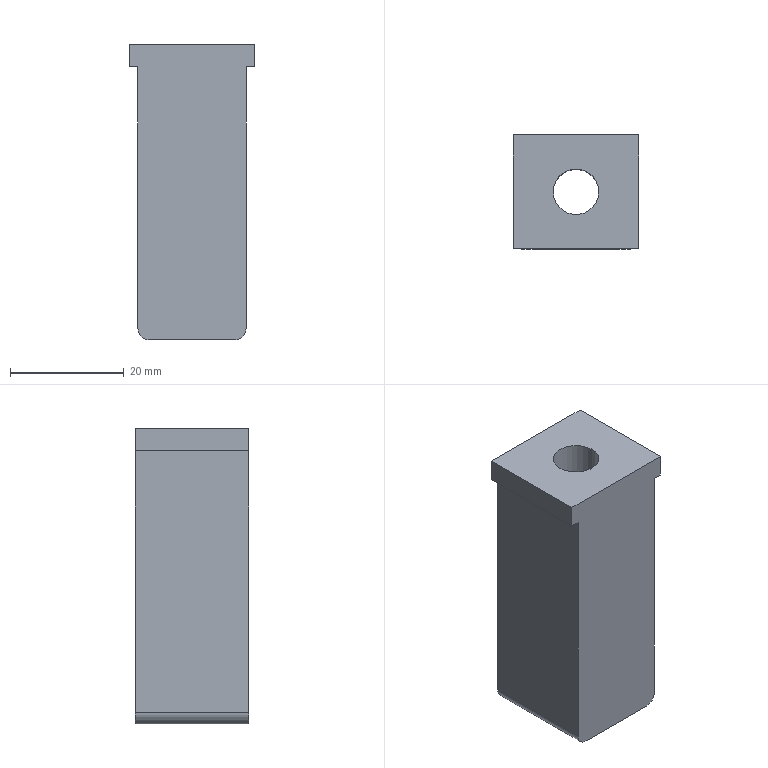Part | NX | features EXTRUDE 3, DATUM_CSYS 2, BLEND 1, SKETCH 1 | 1 solid | 13 faces | box 22 x 20 x 52 mm | volume 17352 mm3 | plane 10 | cylinder 3 | commonest cylinder face diameters 4 x2 8 x1
STEP:
#1=CARTESIAN_POINT('',(9.5,-10.,-50.));
#2=VERTEX_POINT('',#1);
#3=CARTESIAN_POINT('',(9.5,-10.,-4.));
#4=VERTEX_POINT('',#3);
#5=CARTESIAN_POINT('',(9.5,-10.,-52.));
#6=DIRECTION('',(0.,0.,1.));
#7=VECTOR('',#6,1000.);
#8=LINE('',#5,#7);
#9=EDGE_CURVE('',#2,#4,#8,.T.);
#10=ORIENTED_EDGE('',*,*,#9,.F.);
#11=CARTESIAN_POINT('',(9.5,10.,-50.));
#12=VERTEX_POINT('',#11);
#13=CARTESIAN_POINT('',(9.5,10.,-50.));
#14=DIRECTION('',(0.,1.,0.));
#15=VECTOR('',#14,1000.);
#16=LINE('',#13,#15);
#17=EDGE_CURVE('',#2,#12,#16,.T.);
#18=ORIENTED_EDGE('',*,*,#17,.T.);
#19=CARTESIAN_POINT('',(9.5,10.,-4.));
#20=VERTEX_POINT('',#19);
#21=CARTESIAN_POINT('',(9.5,10.,-52.));
#22=DIRECTION('',(0.,0.,1.));
#23=VECTOR('',#22,1000.);
#24=LINE('',#21,#23);
#25=EDGE_CURVE('',#12,#20,#24,.T.);
#26=ORIENTED_EDGE('',*,*,#25,.T.);
#27=CARTESIAN_POINT('',(9.5,-10.,-4.));
#28=DIRECTION('',(0.,1.,0.));
#29=VECTOR('',#28,1000.);
#30=LINE('',#27,#29);
#31=EDGE_CURVE('',#4,#20,#30,.T.);
#32=ORIENTED_EDGE('',*,*,#31,.F.);
#33=EDGE_LOOP('',(#10,#18,#26,#32));
#34=FACE_BOUND('',#33,.T.);
#35=CARTESIAN_POINT('',(9.5,-10.,-52.));
#36=DIRECTION('',(1.,0.,0.));
#37=DIRECTION('',(0.,0.,-1.));
#38=AXIS2_PLACEMENT_3D('',#35,#36,#37);
#39=PLANE('',#38);
#40=ADVANCED_FACE('',(#34),#39,.T.);
#41=ORIENTED_EDGE('',*,*,#25,.F.);
#42=CARTESIAN_POINT('',(7.5,10.,-52.));
#43=VERTEX_POINT('',#42);
#44=CARTESIAN_POINT('',(7.5,10.,-50.));
#45=DIRECTION('',(0.,1.,0.));
#46=DIRECTION('',(0.,0.,1.));
#47=AXIS2_PLACEMENT_3D('',#44,#45,#46);
#48=CIRCLE('',#47,2.);
#49=EDGE_CURVE('',#12,#43,#48,.T.);
#50=ORIENTED_EDGE('',*,*,#49,.T.);
#51=CARTESIAN_POINT('',(-7.5,10.,-52.));
#52=VERTEX_POINT('',#51);
#53=CARTESIAN_POINT('',(9.5,10.,-52.));
#54=DIRECTION('',(-1.,0.,0.));
#55=VECTOR('',#54,1000.);
#56=LINE('',#53,#55);
#57=EDGE_CURVE('',#43,#52,#56,.T.);
#58=ORIENTED_EDGE('',*,*,#57,.T.);
#59=CARTESIAN_POINT('',(-9.5,10.,-50.));
#60=VERTEX_POINT('',#59);
#61=CARTESIAN_POINT('',(-7.5,10.,-50.));
#62=DIRECTION('',(0.,1.,0.));
#63=DIRECTION('',(0.,0.,1.));
#64=AXIS2_PLACEMENT_3D('',#61,#62,#63);
#65=CIRCLE('',#64,2.);
#66=EDGE_CURVE('',#52,#60,#65,.T.);
#67=ORIENTED_EDGE('',*,*,#66,.T.);
#68=CARTESIAN_POINT('',(-9.5,10.,-4.));
#69=VERTEX_POINT('',#68);
#70=CARTESIAN_POINT('',(-9.5,10.,-52.));
#71=DIRECTION('',(0.,0.,1.));
#72=VECTOR('',#71,1000.);
#73=LINE('',#70,#72);
#74=EDGE_CURVE('',#60,#69,#73,.T.);
#75=ORIENTED_EDGE('',*,*,#74,.T.);
#76=CARTESIAN_POINT('',(-11.,10.,-4.));
#77=VERTEX_POINT('',#76);
#78=CARTESIAN_POINT('',(9.5,10.,-4.));
#79=DIRECTION('',(1.,0.,0.));
#80=VECTOR('',#79,1000.);
#81=LINE('',#78,#80);
#82=EDGE_CURVE('',#77,#69,#81,.T.);
#83=ORIENTED_EDGE('',*,*,#82,.F.);
#84=CARTESIAN_POINT('',(-11.,10.,0.));
#85=VERTEX_POINT('',#84);
#86=CARTESIAN_POINT('',(-11.,10.,-4.));
#87=DIRECTION('',(0.,0.,1.));
#88=VECTOR('',#87,1000.);
#89=LINE('',#86,#88);
#90=EDGE_CURVE('',#77,#85,#89,.T.);
#91=ORIENTED_EDGE('',*,*,#90,.T.);
#92=CARTESIAN_POINT('',(11.,10.,0.));
#93=VERTEX_POINT('',#92);
#94=CARTESIAN_POINT('',(9.5,10.,0.));
#95=DIRECTION('',(-1.,0.,0.));
#96=VECTOR('',#95,1000.);
#97=LINE('',#94,#96);
#98=EDGE_CURVE('',#93,#85,#97,.T.);
#99=ORIENTED_EDGE('',*,*,#98,.F.);
#100=CARTESIAN_POINT('',(11.,10.,-4.));
#101=VERTEX_POINT('',#100);
#102=CARTESIAN_POINT('',(11.,10.,-4.));
#103=DIRECTION('',(0.,0.,1.));
#104=VECTOR('',#103,1000.);
#105=LINE('',#102,#104);
#106=EDGE_CURVE('',#101,#93,#105,.T.);
#107=ORIENTED_EDGE('',*,*,#106,.F.);
#108=CARTESIAN_POINT('',(9.5,10.,-4.));
#109=DIRECTION('',(1.,0.,0.));
#110=VECTOR('',#109,1000.);
#111=LINE('',#108,#110);
#112=EDGE_CURVE('',#20,#101,#111,.T.);
#113=ORIENTED_EDGE('',*,*,#112,.F.);
#114=EDGE_LOOP('',(#41,#50,#58,#67,#75,#83,#91,#99,#107,#113));
#115=FACE_BOUND('',#114,.T.);
#116=CARTESIAN_POINT('',(9.5,10.,-52.));
#117=DIRECTION('',(0.,1.,0.));
#118=DIRECTION('',(0.,0.,1.));
#119=AXIS2_PLACEMENT_3D('',#116,#117,#118);
#120=PLANE('',#119);
#121=ADVANCED_FACE('',(#115),#120,.T.);
#122=ORIENTED_EDGE('',*,*,#74,.F.);
#123=CARTESIAN_POINT('',(-9.5,-10.,-50.));
#124=VERTEX_POINT('',#123);
#125=CARTESIAN_POINT('',(-9.5,-10.,-50.));
#126=DIRECTION('',(0.,-1.,0.));
#127=VECTOR('',#126,1000.);
#128=LINE('',#125,#127);
#129=EDGE_CURVE('',#60,#124,#128,.T.);
#130=ORIENTED_EDGE('',*,*,#129,.T.);
#131=CARTESIAN_POINT('',(-9.5,-10.,-4.));
#132=VERTEX_POINT('',#131);
#133=CARTESIAN_POINT('',(-9.5,-10.,-52.));
#134=DIRECTION('',(0.,0.,1.));
#135=VECTOR('',#134,1000.);
#136=LINE('',#133,#135);
#137=EDGE_CURVE('',#124,#132,#136,.T.);
#138=ORIENTED_EDGE('',*,*,#137,.T.);
#139=CARTESIAN_POINT('',(-9.5,10.,-4.));
#140=DIRECTION('',(0.,-1.,0.));
#141=VECTOR('',#140,1000.);
#142=LINE('',#139,#141);
#143=EDGE_CURVE('',#69,#132,#142,.T.);
#144=ORIENTED_EDGE('',*,*,#143,.F.);
#145=EDGE_LOOP('',(#122,#130,#138,#144));
#146=FACE_BOUND('',#145,.T.);
#147=CARTESIAN_POINT('',(-9.5,10.,-52.));
#148=DIRECTION('',(-1.,0.,0.));
#149=DIRECTION('',(0.,0.,1.));
#150=AXIS2_PLACEMENT_3D('',#147,#148,#149);
#151=PLANE('',#150);
#152=ADVANCED_FACE('',(#146),#151,.T.);
#153=CARTESIAN_POINT('',(-7.5,-10.,-52.));
#154=VERTEX_POINT('',#153);
#155=CARTESIAN_POINT('',(7.5,-10.,-52.));
#156=VERTEX_POINT('',#155);
#157=CARTESIAN_POINT('',(-9.5,-10.,-52.));
#158=DIRECTION('',(1.,0.,0.));
#159=VECTOR('',#158,1000.);
#160=LINE('',#157,#159);
#161=EDGE_CURVE('',#154,#156,#160,.T.);
#162=ORIENTED_EDGE('',*,*,#161,.T.);
#163=CARTESIAN_POINT('',(7.5,-10.,-50.));
#164=DIRECTION('',(0.,-1.,0.));
#165=DIRECTION('',(1.,0.,0.));
#166=AXIS2_PLACEMENT_3D('',#163,#164,#165);
#167=CIRCLE('',#166,2.);
#168=EDGE_CURVE('',#156,#2,#167,.T.);
#169=ORIENTED_EDGE('',*,*,#168,.T.);
#170=ORIENTED_EDGE('',*,*,#9,.T.);
#171=CARTESIAN_POINT('',(11.,-10.,-4.));
#172=VERTEX_POINT('',#171);
#173=CARTESIAN_POINT('',(11.,-10.,-4.));
#174=DIRECTION('',(-1.,0.,0.));
#175=VECTOR('',#174,1000.);
#176=LINE('',#173,#175);
#177=EDGE_CURVE('',#172,#4,#176,.T.);
#178=ORIENTED_EDGE('',*,*,#177,.F.);
#179=CARTESIAN_POINT('',(11.,-10.,0.));
#180=VERTEX_POINT('',#179);
#181=CARTESIAN_POINT('',(11.,-10.,-4.));
#182=DIRECTION('',(0.,0.,1.));
#183=VECTOR('',#182,1000.);
#184=LINE('',#181,#183);
#185=EDGE_CURVE('',#172,#180,#184,.T.);
#186=ORIENTED_EDGE('',*,*,#185,.T.);
#187=CARTESIAN_POINT('',(-11.,-10.,0.));
#188=VERTEX_POINT('',#187);
#189=CARTESIAN_POINT('',(-9.5,-10.,0.));
#190=DIRECTION('',(1.,0.,0.));
#191=VECTOR('',#190,1000.);
#192=LINE('',#189,#191);
#193=EDGE_CURVE('',#188,#180,#192,.T.);
#194=ORIENTED_EDGE('',*,*,#193,.F.);
#195=CARTESIAN_POINT('',(-11.,-10.,-4.));
#196=VERTEX_POINT('',#195);
#197=CARTESIAN_POINT('',(-11.,-10.,-4.));
#198=DIRECTION('',(0.,0.,1.));
#199=VECTOR('',#198,1000.);
#200=LINE('',#197,#199);
#201=EDGE_CURVE('',#196,#188,#200,.T.);
#202=ORIENTED_EDGE('',*,*,#201,.F.);
#203=CARTESIAN_POINT('',(11.,-10.,-4.));
#204=DIRECTION('',(-1.,0.,0.));
#205=VECTOR('',#204,1000.);
#206=LINE('',#203,#205);
#207=EDGE_CURVE('',#132,#196,#206,.T.);
#208=ORIENTED_EDGE('',*,*,#207,.F.);
#209=ORIENTED_EDGE('',*,*,#137,.F.);
#210=CARTESIAN_POINT('',(-7.5,-10.,-50.));
#211=DIRECTION('',(0.,-1.,0.));
#212=DIRECTION('',(1.,0.,0.));
#213=AXIS2_PLACEMENT_3D('',#210,#211,#212);
#214=CIRCLE('',#213,2.);
#215=EDGE_CURVE('',#124,#154,#214,.T.);
#216=ORIENTED_EDGE('',*,*,#215,.T.);
#217=EDGE_LOOP('',(#162,#169,#170,#178,#186,#194,#202,#208,#209,#216));
#218=FACE_BOUND('',#217,.T.);
#219=CARTESIAN_POINT('',(-9.5,-10.,-52.));
#220=DIRECTION('',(0.,-1.,0.));
#221=DIRECTION('',(1.,0.,0.));
#222=AXIS2_PLACEMENT_3D('',#219,#220,#221);
#223=PLANE('',#222);
#224=ADVANCED_FACE('',(#218),#223,.T.);
#225=CARTESIAN_POINT('',(4.,0.,-52.));
#226=VERTEX_POINT('',#225);
#227=CARTESIAN_POINT('',(0.,0.,-52.));
#228=DIRECTION('',(0.,0.,1.));
#229=DIRECTION('',(1.,0.,0.));
#230=AXIS2_PLACEMENT_3D('',#227,#228,#229);
#231=CIRCLE('',#230,4.);
#232=EDGE_CURVE('',#226,#226,#231,.T.);
#233=ORIENTED_EDGE('',*,*,#232,.T.);
#234=EDGE_LOOP('',(#233));
#235=FACE_BOUND('',#234,.T.);
#236=ORIENTED_EDGE('',*,*,#57,.F.);
#237=CARTESIAN_POINT('',(7.5,-10.,-52.));
#238=DIRECTION('',(0.,1.,0.));
#239=VECTOR('',#238,1000.);
#240=LINE('',#237,#239);
#241=EDGE_CURVE('',#43,#156,#240,.F.);
#242=ORIENTED_EDGE('',*,*,#241,.T.);
#243=ORIENTED_EDGE('',*,*,#161,.F.);
#244=CARTESIAN_POINT('',(-7.5,10.,-52.));
#245=DIRECTION('',(0.,-1.,0.));
#246=VECTOR('',#245,1000.);
#247=LINE('',#244,#246);
#248=EDGE_CURVE('',#154,#52,#247,.F.);
#249=ORIENTED_EDGE('',*,*,#248,.T.);
#250=EDGE_LOOP('',(#236,#242,#243,#249));
#251=FACE_BOUND('',#250,.T.);
#252=CARTESIAN_POINT('',(0.,0.,-52.));
#253=DIRECTION('',(0.,0.,1.));
#254=DIRECTION('',(1.,0.,0.));
#255=AXIS2_PLACEMENT_3D('',#252,#253,#254);
#256=PLANE('',#255);
#257=ADVANCED_FACE('',(#235,#251),#256,.F.);
#258=CARTESIAN_POINT('',(4.,0.,0.));
#259=VERTEX_POINT('',#258);
#260=CARTESIAN_POINT('',(0.,0.,0.));
#261=DIRECTION('',(0.,0.,1.));
#262=DIRECTION('',(1.,0.,0.));
#263=AXIS2_PLACEMENT_3D('',#260,#261,#262);
#264=CIRCLE('',#263,4.);
#265=EDGE_CURVE('',#259,#259,#264,.T.);
#266=ORIENTED_EDGE('',*,*,#265,.F.);
#267=EDGE_LOOP('',(#266));
#268=FACE_BOUND('',#267,.T.);
#269=ORIENTED_EDGE('',*,*,#193,.T.);
#270=CARTESIAN_POINT('',(11.,10.,0.));
#271=DIRECTION('',(0.,-1.,0.));
#272=VECTOR('',#271,1000.);
#273=LINE('',#270,#272);
#274=EDGE_CURVE('',#93,#180,#273,.T.);
#275=ORIENTED_EDGE('',*,*,#274,.F.);
#276=ORIENTED_EDGE('',*,*,#98,.T.);
#277=CARTESIAN_POINT('',(-11.,-10.,0.));
#278=DIRECTION('',(0.,1.,0.));
#279=VECTOR('',#278,1000.);
#280=LINE('',#277,#279);
#281=EDGE_CURVE('',#188,#85,#280,.T.);
#282=ORIENTED_EDGE('',*,*,#281,.F.);
#283=EDGE_LOOP('',(#269,#275,#276,#282));
#284=FACE_BOUND('',#283,.T.);
#285=CARTESIAN_POINT('',(0.,0.,0.));
#286=DIRECTION('',(0.,0.,1.));
#287=DIRECTION('',(1.,0.,0.));
#288=AXIS2_PLACEMENT_3D('',#285,#286,#287);
#289=PLANE('',#288);
#290=ADVANCED_FACE('',(#268,#284),#289,.T.);
#291=ORIENTED_EDGE('',*,*,#281,.T.);
#292=ORIENTED_EDGE('',*,*,#90,.F.);
#293=CARTESIAN_POINT('',(-11.,-10.,-4.));
#294=DIRECTION('',(0.,1.,0.));
#295=VECTOR('',#294,1000.);
#296=LINE('',#293,#295);
#297=EDGE_CURVE('',#196,#77,#296,.T.);
#298=ORIENTED_EDGE('',*,*,#297,.F.);
#299=ORIENTED_EDGE('',*,*,#201,.T.);
#300=EDGE_LOOP('',(#291,#292,#298,#299));
#301=FACE_BOUND('',#300,.T.);
#302=CARTESIAN_POINT('',(-11.,-10.,-4.));
#303=DIRECTION('',(1.,0.,0.));
#304=DIRECTION('',(0.,0.,-1.));
#305=AXIS2_PLACEMENT_3D('',#302,#303,#304);
#306=PLANE('',#305);
#307=ADVANCED_FACE('',(#301),#306,.F.);
#308=ORIENTED_EDGE('',*,*,#82,.T.);
#309=ORIENTED_EDGE('',*,*,#143,.T.);
#310=ORIENTED_EDGE('',*,*,#207,.T.);
#311=ORIENTED_EDGE('',*,*,#297,.T.);
#312=EDGE_LOOP('',(#308,#309,#310,#311));
#313=FACE_BOUND('',#312,.T.);
#314=CARTESIAN_POINT('',(0.,0.,-4.));
#315=DIRECTION('',(0.,0.,-1.));
#316=DIRECTION('',(-1.,0.,0.));
#317=AXIS2_PLACEMENT_3D('',#314,#315,#316);
#318=PLANE('',#317);
#319=ADVANCED_FACE('',(#313),#318,.T.);
#320=ORIENTED_EDGE('',*,*,#177,.T.);
#321=ORIENTED_EDGE('',*,*,#31,.T.);
#322=ORIENTED_EDGE('',*,*,#112,.T.);
#323=CARTESIAN_POINT('',(11.,10.,-4.));
#324=DIRECTION('',(0.,-1.,0.));
#325=VECTOR('',#324,1000.);
#326=LINE('',#323,#325);
#327=EDGE_CURVE('',#101,#172,#326,.T.);
#328=ORIENTED_EDGE('',*,*,#327,.T.);
#329=EDGE_LOOP('',(#320,#321,#322,#328));
#330=FACE_BOUND('',#329,.T.);
#331=CARTESIAN_POINT('',(0.,0.,-4.));
#332=DIRECTION('',(0.,0.,-1.));
#333=DIRECTION('',(-1.,0.,0.));
#334=AXIS2_PLACEMENT_3D('',#331,#332,#333);
#335=PLANE('',#334);
#336=ADVANCED_FACE('',(#330),#335,.T.);
#337=ORIENTED_EDGE('',*,*,#274,.T.);
#338=ORIENTED_EDGE('',*,*,#185,.F.);
#339=ORIENTED_EDGE('',*,*,#327,.F.);
#340=ORIENTED_EDGE('',*,*,#106,.T.);
#341=EDGE_LOOP('',(#337,#338,#339,#340));
#342=FACE_BOUND('',#341,.T.);
#343=CARTESIAN_POINT('',(11.,10.,-4.));
#344=DIRECTION('',(-1.,0.,0.));
#345=DIRECTION('',(0.,0.,1.));
#346=AXIS2_PLACEMENT_3D('',#343,#344,#345);
#347=PLANE('',#346);
#348=ADVANCED_FACE('',(#342),#347,.F.);
#349=ORIENTED_EDGE('',*,*,#265,.T.);
#350=EDGE_LOOP('',(#349));
#351=FACE_BOUND('',#350,.T.);
#352=ORIENTED_EDGE('',*,*,#232,.F.);
#353=EDGE_LOOP('',(#352));
#354=FACE_BOUND('',#353,.T.);
#355=CARTESIAN_POINT('',(0.,0.,-57.2));
#356=DIRECTION('',(0.,0.,1.));
#357=DIRECTION('',(1.,0.,0.));
#358=AXIS2_PLACEMENT_3D('',#355,#356,#357);
#359=CYLINDRICAL_SURFACE('',#358,4.);
#360=ADVANCED_FACE('',(#351,#354),#359,.F.);
#361=ORIENTED_EDGE('',*,*,#168,.F.);
#362=ORIENTED_EDGE('',*,*,#241,.F.);
#363=ORIENTED_EDGE('',*,*,#49,.F.);
#364=ORIENTED_EDGE('',*,*,#17,.F.);
#365=EDGE_LOOP('',(#361,#362,#363,#364));
#366=FACE_BOUND('',#365,.T.);
#367=CARTESIAN_POINT('',(7.5,-10.,-50.));
#368=DIRECTION('',(0.,-1.,0.));
#369=DIRECTION('',(0.,0.,-1.));
#370=AXIS2_PLACEMENT_3D('',#367,#368,#369);
#371=CYLINDRICAL_SURFACE('',#370,2.);
#372=ADVANCED_FACE('',(#366),#371,.T.);
#373=ORIENTED_EDGE('',*,*,#66,.F.);
#374=ORIENTED_EDGE('',*,*,#248,.F.);
#375=ORIENTED_EDGE('',*,*,#215,.F.);
#376=ORIENTED_EDGE('',*,*,#129,.F.);
#377=EDGE_LOOP('',(#373,#374,#375,#376));
#378=FACE_BOUND('',#377,.T.);
#379=CARTESIAN_POINT('',(-7.5,10.,-50.));
#380=DIRECTION('',(0.,1.,0.));
#381=DIRECTION('',(0.,0.,1.));
#382=AXIS2_PLACEMENT_3D('',#379,#380,#381);
#383=CYLINDRICAL_SURFACE('',#382,2.);
#384=ADVANCED_FACE('',(#378),#383,.T.);
#385=CLOSED_SHELL('',(#40,#121,#152,#224,#257,#290,#307,#319,#336,#348,#360,#372,#384));
#386=MANIFOLD_SOLID_BREP('',#385);
#387=(LENGTH_UNIT()NAMED_UNIT(*)SI_UNIT(.MILLI.,.METRE.));
#388=UNCERTAINTY_MEASURE_WITH_UNIT(LENGTH_MEASURE(0.00001),#387,'','');
#389=(NAMED_UNIT(*)PLANE_ANGLE_UNIT()SI_UNIT($,.RADIAN.));
#390=(NAMED_UNIT(*)SI_UNIT($,.STERADIAN.)SOLID_ANGLE_UNIT());
#391=(GEOMETRIC_REPRESENTATION_CONTEXT(3)GLOBAL_UNCERTAINTY_ASSIGNED_CONTEXT((#388))GLOBAL_UNIT_ASSIGNED_CONTEXT((#387,#389,#390))REPRESENTATION_CONTEXT('',''));
#392=ADVANCED_BREP_SHAPE_REPRESENTATION('',(#386),#391);